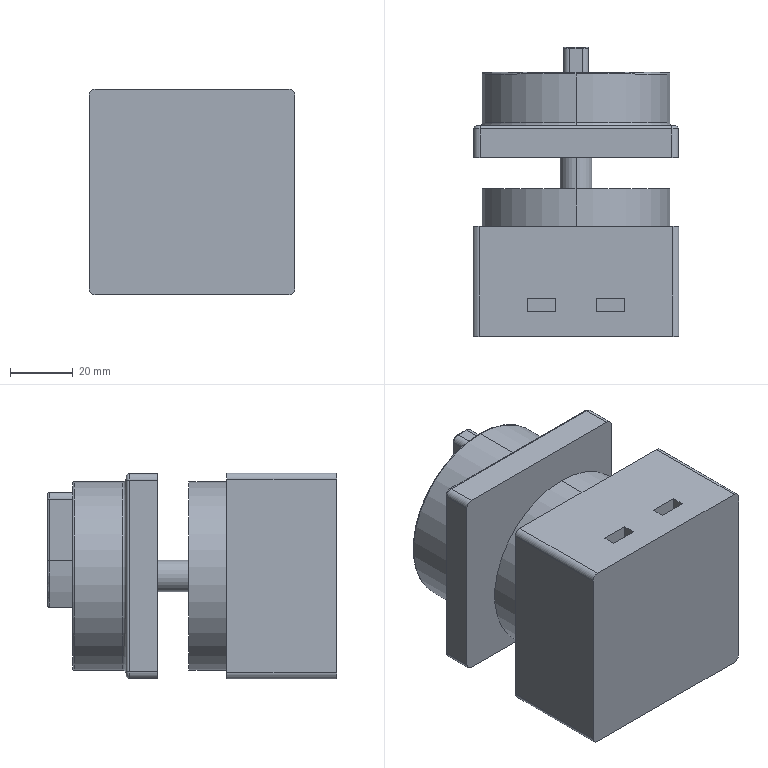Part | STEP file | Power switch LW42B2-1824_L | 1 solid | 95 faces | box 65.5 x 92 x 65.5 mm | volume 250369 mm3 | plane 43 | cylinder 36 | torus 13 | spline 2 | other 1 | commonest cylinder face diameters 4 x10 2 x6 1 x4 4.5 x4 60 x4 0.4 x2